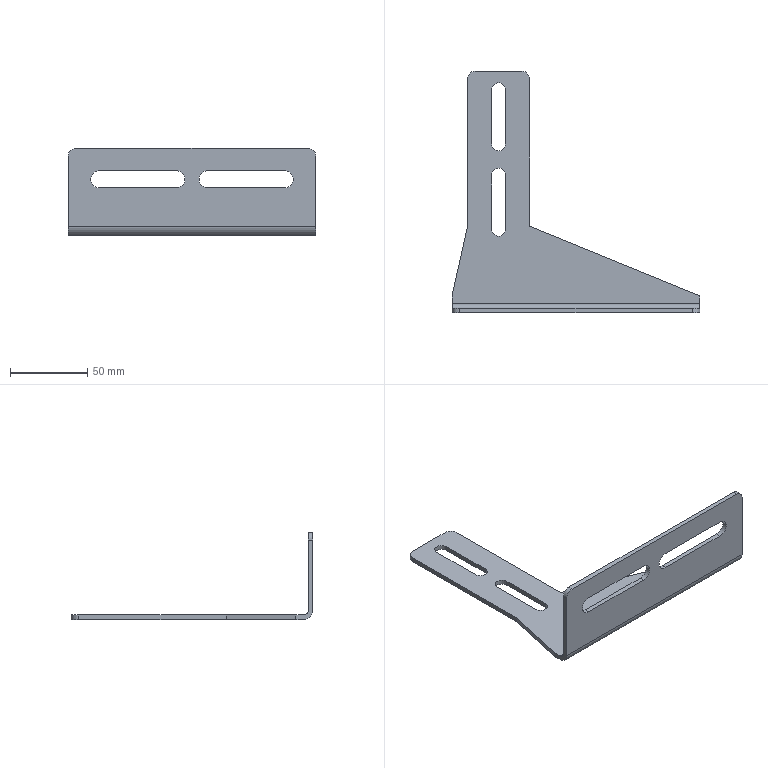Part | STEP file | Sheet29 | 1 solid | 34 faces | box 160 x 156 x 56.288 mm | volume 49225 mm3 | plane 20 | cylinder 14 | commonest cylinder face diameters 9 x4 10 x4 11 x4 6 x1 12 x1